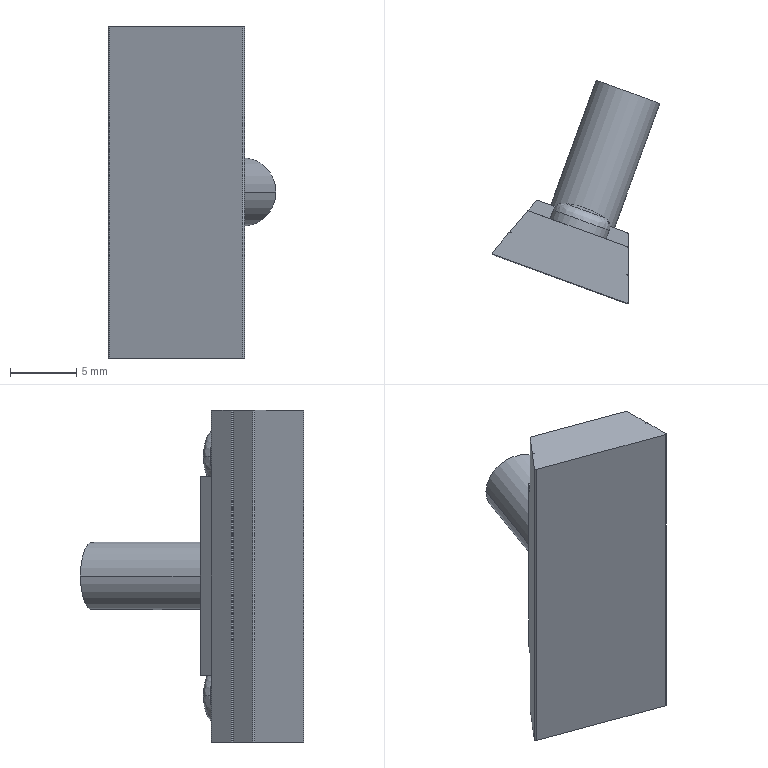Part | SolidWorks | features BaseBody 1 | 1 solid | 43 faces | box 12.626 x 16.806 x 25 mm | volume 1310 mm3 | plane 19 | cylinder 18 | spline 6 | commonest cylinder face diameters 0.2 x10 4.5 x4 5 x2 5.1 x2
STEP:
#1=CARTESIAN_POINT('',(0.2959,5.705,-9.));
#2=VERTEX_POINT('',#1);
#3=CARTESIAN_POINT('',(3.44,4.56,-9.));
#4=VERTEX_POINT('',#3);
#5=CARTESIAN_POINT('',(1.868,5.133,-9.));
#6=DIRECTION('',(-0.342,-0.9397,0.));
#7=DIRECTION('',(-0.9397,0.342,0.));
#8=AXIS2_PLACEMENT_3D('',#5,#6,#7);
#9=CIRCLE('',#8,1.673);
#10=EDGE_CURVE('',#2,#4,#9,.T.);
#11=ORIENTED_EDGE('',*,*,#10,.T.);
#12=CARTESIAN_POINT('',(3.72,3.641,-9.));
#13=VERTEX_POINT('',#12);
#14=CARTESIAN_POINT('',(2.968,3.915,-9.));
#15=DIRECTION('',(0.,0.,-1.));
#16=DIRECTION('',(0.9397,-0.342,0.));
#17=AXIS2_PLACEMENT_3D('',#14,#15,#16);
#18=CIRCLE('',#17,0.8);
#19=EDGE_CURVE('',#4,#13,#18,.T.);
#20=ORIENTED_EDGE('',*,*,#19,.T.);
#21=CARTESIAN_POINT('',(-0.509,5.18,-9.));
#22=VERTEX_POINT('',#21);
#23=CARTESIAN_POINT('',(1.605,4.411,-9.));
#24=DIRECTION('',(-0.342,-0.9397,0.));
#25=DIRECTION('',(0.9397,-0.342,0.));
#26=AXIS2_PLACEMENT_3D('',#23,#24,#25);
#27=CIRCLE('',#26,2.25);
#28=EDGE_CURVE('',#22,#13,#27,.T.);
#29=ORIENTED_EDGE('',*,*,#28,.F.);
#30=CARTESIAN_POINT('',(0.2428,4.907,-9.));
#31=DIRECTION('',(0.,0.,1.));
#32=DIRECTION('',(-0.9397,0.342,0.));
#33=AXIS2_PLACEMENT_3D('',#30,#31,#32);
#34=CIRCLE('',#33,0.8);
#35=EDGE_CURVE('',#2,#22,#34,.T.);
#36=ORIENTED_EDGE('',*,*,#35,.F.);
#37=EDGE_LOOP('',(#11,#20,#29,#36));
#38=FACE_OUTER_BOUND('',#37,.T.);
#39=CARTESIAN_POINT('',(3.44,4.56,-9.));
#40=CARTESIAN_POINT('',(3.44,4.56,-12.346));
#41=CARTESIAN_POINT('',(0.2959,5.705,-12.346));
#42=CARTESIAN_POINT('',(0.2959,5.705,-9.));
#43=CARTESIAN_POINT('',(3.739,4.342,-9.));
#44=CARTESIAN_POINT('',(3.739,4.342,-13.056));
#45=CARTESIAN_POINT('',(-0.07287,5.729,-13.056));
#46=CARTESIAN_POINT('',(-0.07287,5.729,-9.));
#47=CARTESIAN_POINT('',(3.846,3.988,-9.));
#48=CARTESIAN_POINT('',(3.846,3.988,-13.5));
#49=CARTESIAN_POINT('',(-0.3825,5.528,-13.5));
#50=CARTESIAN_POINT('',(-0.3825,5.528,-9.));
#51=CARTESIAN_POINT('',(3.72,3.641,-9.));
#52=CARTESIAN_POINT('',(3.72,3.641,-13.5));
#53=CARTESIAN_POINT('',(-0.509,5.18,-13.5));
#54=CARTESIAN_POINT('',(-0.509,5.18,-9.));
#55=(BOUNDED_SURFACE()B_SPLINE_SURFACE(3,3,((#39,#40,#41,#42),(#43,#44,#45,#46),(#47,#48,#49,#50),(#51,#52,#53,#54)),.UNSPECIFIED.,.F.,.F.,.T.)B_SPLINE_SURFACE_WITH_KNOTS((4,4),(4,4),(0.,1.),(0.,1.),.UNSPECIFIED.)GEOMETRIC_REPRESENTATION_ITEM()RATIONAL_B_SPLINE_SURFACE(((1.,0.3333,0.3333,1.),(0.8664,0.2888,0.2888,0.8664),(0.8664,0.2888,0.2888,0.8664),(1.,0.3333,0.3333,1.)))REPRESENTATION_ITEM('')SURFACE());
#56=ADVANCED_FACE('',(#38),#55,.T.);
#57=CARTESIAN_POINT('',(0.2959,5.705,9.));
#58=VERTEX_POINT('',#57);
#59=CARTESIAN_POINT('',(3.44,4.56,9.));
#60=VERTEX_POINT('',#59);
#61=CARTESIAN_POINT('',(1.868,5.133,9.));
#62=DIRECTION('',(-0.342,-0.9397,0.));
#63=DIRECTION('',(-0.9397,0.342,0.));
#64=AXIS2_PLACEMENT_3D('',#61,#62,#63);
#65=CIRCLE('',#64,1.673);
#66=EDGE_CURVE('',#58,#60,#65,.T.);
#67=ORIENTED_EDGE('',*,*,#66,.T.);
#68=CARTESIAN_POINT('',(3.72,3.641,9.));
#69=VERTEX_POINT('',#68);
#70=CARTESIAN_POINT('',(2.968,3.915,9.));
#71=DIRECTION('',(0.,0.,-1.));
#72=DIRECTION('',(0.9397,-0.342,0.));
#73=AXIS2_PLACEMENT_3D('',#70,#71,#72);
#74=CIRCLE('',#73,0.8);
#75=EDGE_CURVE('',#60,#69,#74,.T.);
#76=ORIENTED_EDGE('',*,*,#75,.T.);
#77=CARTESIAN_POINT('',(-0.509,5.18,9.));
#78=VERTEX_POINT('',#77);
#79=CARTESIAN_POINT('',(1.605,4.411,9.));
#80=DIRECTION('',(-0.342,-0.9397,0.));
#81=DIRECTION('',(0.9397,-0.342,0.));
#82=AXIS2_PLACEMENT_3D('',#79,#80,#81);
#83=CIRCLE('',#82,2.25);
#84=EDGE_CURVE('',#78,#69,#83,.T.);
#85=ORIENTED_EDGE('',*,*,#84,.F.);
#86=CARTESIAN_POINT('',(0.2428,4.907,9.));
#87=DIRECTION('',(0.,0.,1.));
#88=DIRECTION('',(-0.9397,0.342,0.));
#89=AXIS2_PLACEMENT_3D('',#86,#87,#88);
#90=CIRCLE('',#89,0.8);
#91=EDGE_CURVE('',#58,#78,#90,.T.);
#92=ORIENTED_EDGE('',*,*,#91,.F.);
#93=EDGE_LOOP('',(#67,#76,#85,#92));
#94=FACE_OUTER_BOUND('',#93,.T.);
#95=CARTESIAN_POINT('',(3.44,4.56,9.));
#96=CARTESIAN_POINT('',(3.44,4.56,5.654));
#97=CARTESIAN_POINT('',(0.2959,5.705,5.654));
#98=CARTESIAN_POINT('',(0.2959,5.705,9.));
#99=CARTESIAN_POINT('',(3.739,4.342,9.));
#100=CARTESIAN_POINT('',(3.739,4.342,4.944));
#101=CARTESIAN_POINT('',(-0.07287,5.729,4.944));
#102=CARTESIAN_POINT('',(-0.07287,5.729,9.));
#103=CARTESIAN_POINT('',(3.846,3.988,9.));
#104=CARTESIAN_POINT('',(3.846,3.988,4.5));
#105=CARTESIAN_POINT('',(-0.3825,5.528,4.5));
#106=CARTESIAN_POINT('',(-0.3825,5.528,9.));
#107=CARTESIAN_POINT('',(3.72,3.641,9.));
#108=CARTESIAN_POINT('',(3.72,3.641,4.5));
#109=CARTESIAN_POINT('',(-0.509,5.18,4.5));
#110=CARTESIAN_POINT('',(-0.509,5.18,9.));
#111=(BOUNDED_SURFACE()B_SPLINE_SURFACE(3,3,((#95,#96,#97,#98),(#99,#100,#101,#102),(#103,#104,#105,#106),(#107,#108,#109,#110)),.UNSPECIFIED.,.F.,.F.,.T.)B_SPLINE_SURFACE_WITH_KNOTS((4,4),(4,4),(0.,1.),(0.,1.),.UNSPECIFIED.)GEOMETRIC_REPRESENTATION_ITEM()RATIONAL_B_SPLINE_SURFACE(((1.,0.3333,0.3333,1.),(0.8664,0.2888,0.2888,0.8664),(0.8664,0.2888,0.2888,0.8664),(1.,0.3333,0.3333,1.)))REPRESENTATION_ITEM('')SURFACE());
#112=ADVANCED_FACE('',(#94),#111,.T.);
#113=CARTESIAN_POINT('',(1.605,4.411,-9.));
#114=DIRECTION('',(-0.342,-0.9397,0.));
#115=DIRECTION('',(0.9397,-0.342,0.));
#116=AXIS2_PLACEMENT_3D('',#113,#114,#115);
#117=CIRCLE('',#116,2.25);
#118=EDGE_CURVE('',#13,#22,#117,.T.);
#119=ORIENTED_EDGE('',*,*,#118,.T.);
#120=CARTESIAN_POINT('',(-0.7462,4.528,-9.));
#121=VERTEX_POINT('',#120);
#122=CARTESIAN_POINT('',(-0.1648,6.126,-9.));
#123=DIRECTION('',(-0.342,-0.9397,0.));
#124=VECTOR('',#123,1000.);
#125=LINE('',#122,#124);
#126=EDGE_CURVE('',#22,#121,#125,.T.);
#127=ORIENTED_EDGE('',*,*,#126,.T.);
#128=CARTESIAN_POINT('',(3.482,2.989,-9.));
#129=VERTEX_POINT('',#128);
#130=CARTESIAN_POINT('',(1.368,3.759,-9.));
#131=DIRECTION('',(0.342,0.9397,0.));
#132=DIRECTION('',(0.9397,-0.342,0.));
#133=AXIS2_PLACEMENT_3D('',#130,#131,#132);
#134=CIRCLE('',#133,2.25);
#135=EDGE_CURVE('',#121,#129,#134,.T.);
#136=ORIENTED_EDGE('',*,*,#135,.T.);
#137=CARTESIAN_POINT('',(4.064,4.587,-9.));
#138=DIRECTION('',(-0.342,-0.9397,0.));
#139=VECTOR('',#138,1000.);
#140=LINE('',#137,#139);
#141=EDGE_CURVE('',#13,#129,#140,.T.);
#142=ORIENTED_EDGE('',*,*,#141,.F.);
#143=EDGE_LOOP('',(#119,#127,#136,#142));
#144=FACE_OUTER_BOUND('',#143,.T.);
#145=CARTESIAN_POINT('',(1.95,5.356,-9.));
#146=DIRECTION('',(-0.342,-0.9397,0.));
#147=DIRECTION('',(0.9397,-0.342,0.));
#148=AXIS2_PLACEMENT_3D('',#145,#146,#147);
#149=CYLINDRICAL_SURFACE('',#148,2.25);
#150=ADVANCED_FACE('',(#144),#149,.T.);
#151=CARTESIAN_POINT('',(1.605,4.411,9.));
#152=DIRECTION('',(-0.342,-0.9397,0.));
#153=DIRECTION('',(0.9397,-0.342,0.));
#154=AXIS2_PLACEMENT_3D('',#151,#152,#153);
#155=CIRCLE('',#154,2.25);
#156=EDGE_CURVE('',#69,#78,#155,.T.);
#157=ORIENTED_EDGE('',*,*,#156,.T.);
#158=CARTESIAN_POINT('',(-0.7462,4.528,9.));
#159=VERTEX_POINT('',#158);
#160=CARTESIAN_POINT('',(-0.1648,6.126,9.));
#161=DIRECTION('',(-0.342,-0.9397,0.));
#162=VECTOR('',#161,1000.);
#163=LINE('',#160,#162);
#164=EDGE_CURVE('',#78,#159,#163,.T.);
#165=ORIENTED_EDGE('',*,*,#164,.T.);
#166=CARTESIAN_POINT('',(3.482,2.989,9.));
#167=VERTEX_POINT('',#166);
#168=CARTESIAN_POINT('',(1.368,3.759,9.));
#169=DIRECTION('',(0.342,0.9397,0.));
#170=DIRECTION('',(0.9397,-0.342,0.));
#171=AXIS2_PLACEMENT_3D('',#168,#169,#170);
#172=CIRCLE('',#171,2.25);
#173=EDGE_CURVE('',#159,#167,#172,.T.);
#174=ORIENTED_EDGE('',*,*,#173,.T.);
#175=CARTESIAN_POINT('',(4.064,4.587,9.));
#176=DIRECTION('',(-0.342,-0.9397,0.));
#177=VECTOR('',#176,1000.);
#178=LINE('',#175,#177);
#179=EDGE_CURVE('',#69,#167,#178,.T.);
#180=ORIENTED_EDGE('',*,*,#179,.F.);
#181=EDGE_LOOP('',(#157,#165,#174,#180));
#182=FACE_OUTER_BOUND('',#181,.T.);
#183=CARTESIAN_POINT('',(1.95,5.356,9.));
#184=DIRECTION('',(-0.342,-0.9397,0.));
#185=DIRECTION('',(0.9397,-0.342,0.));
#186=AXIS2_PLACEMENT_3D('',#183,#184,#185);
#187=CYLINDRICAL_SURFACE('',#186,2.25);
#188=ADVANCED_FACE('',(#182),#187,.T.);
#189=CARTESIAN_POINT('',(-0.6861,5.571,0.));
#190=VERTEX_POINT('',#189);
#191=CARTESIAN_POINT('',(4.106,3.826,0.));
#192=VERTEX_POINT('',#191);
#193=CARTESIAN_POINT('',(1.71,4.698,0.));
#194=DIRECTION('',(0.342,0.9397,0.));
#195=DIRECTION('',(-0.9397,0.342,0.));
#196=AXIS2_PLACEMENT_3D('',#193,#194,#195);
#197=CIRCLE('',#196,2.55);
#198=EDGE_CURVE('',#190,#192,#197,.T.);
#199=ORIENTED_EDGE('',*,*,#198,.T.);
#200=CARTESIAN_POINT('',(7.527,13.223,0.));
#201=VERTEX_POINT('',#200);
#202=CARTESIAN_POINT('',(7.527,13.223,0.));
#203=DIRECTION('',(0.342,0.9397,0.));
#204=VECTOR('',#203,1000.);
#205=LINE('',#202,#204);
#206=EDGE_CURVE('',#192,#201,#205,.T.);
#207=ORIENTED_EDGE('',*,*,#206,.T.);
#208=CARTESIAN_POINT('',(2.734,14.968,0.));
#209=VERTEX_POINT('',#208);
#210=CARTESIAN_POINT('',(5.13,14.095,0.));
#211=DIRECTION('',(-0.342,-0.9397,0.));
#212=DIRECTION('',(-0.9397,0.342,0.));
#213=AXIS2_PLACEMENT_3D('',#210,#211,#212);
#214=CIRCLE('',#213,2.55);
#215=EDGE_CURVE('',#201,#209,#214,.T.);
#216=ORIENTED_EDGE('',*,*,#215,.T.);
#217=CARTESIAN_POINT('',(2.734,14.968,0.));
#218=DIRECTION('',(0.342,0.9397,0.));
#219=VECTOR('',#218,1000.);
#220=LINE('',#217,#219);
#221=EDGE_CURVE('',#190,#209,#220,.T.);
#222=ORIENTED_EDGE('',*,*,#221,.F.);
#223=EDGE_LOOP('',(#199,#207,#216,#222));
#224=FACE_OUTER_BOUND('',#223,.T.);
#225=CARTESIAN_POINT('',(5.13,14.095,0.));
#226=DIRECTION('',(0.342,0.9397,0.));
#227=DIRECTION('',(-0.9397,0.342,0.));
#228=AXIS2_PLACEMENT_3D('',#225,#226,#227);
#229=CYLINDRICAL_SURFACE('',#228,2.55);
#230=ADVANCED_FACE('',(#224),#229,.T.);
#231=CARTESIAN_POINT('',(5.034,-1.832,12.5));
#232=VERTEX_POINT('',#231);
#233=CARTESIAN_POINT('',(5.034,-1.832,-12.5));
#234=VERTEX_POINT('',#233);
#235=CARTESIAN_POINT('',(5.034,-1.832,12.5));
#236=DIRECTION('',(0.,0.,-1.));
#237=VECTOR('',#236,1000.);
#238=LINE('',#235,#237);
#239=EDGE_CURVE('',#232,#234,#238,.T.);
#240=ORIENTED_EDGE('',*,*,#239,.F.);
#241=CARTESIAN_POINT('',(-5.034,1.832,12.5));
#242=VERTEX_POINT('',#241);
#243=CARTESIAN_POINT('',(-5.034,1.832,12.5));
#244=DIRECTION('',(0.9397,-0.342,0.));
#245=VECTOR('',#244,1000.);
#246=LINE('',#243,#245);
#247=EDGE_CURVE('',#242,#232,#246,.T.);
#248=ORIENTED_EDGE('',*,*,#247,.F.);
#249=CARTESIAN_POINT('',(-5.034,1.832,-12.5));
#250=VERTEX_POINT('',#249);
#251=CARTESIAN_POINT('',(-5.034,1.832,12.5));
#252=DIRECTION('',(0.,0.,1.));
#253=VECTOR('',#252,1000.);
#254=LINE('',#251,#253);
#255=EDGE_CURVE('',#250,#242,#254,.T.);
#256=ORIENTED_EDGE('',*,*,#255,.F.);
#257=CARTESIAN_POINT('',(-5.034,1.832,-12.5));
#258=DIRECTION('',(-0.9397,0.342,0.));
#259=VECTOR('',#258,1000.);
#260=LINE('',#257,#259);
#261=EDGE_CURVE('',#234,#250,#260,.T.);
#262=ORIENTED_EDGE('',*,*,#261,.F.);
#263=EDGE_LOOP('',(#240,#248,#256,#262));
#264=FACE_OUTER_BOUND('',#263,.T.);
#265=CARTESIAN_POINT('',(-5.034,1.832,12.5));
#266=DIRECTION('',(0.342,0.9397,0.));
#267=DIRECTION('',(-0.9397,0.342,0.));
#268=AXIS2_PLACEMENT_3D('',#265,#266,#267);
#269=PLANE('',#268);
#270=ADVANCED_FACE('',(#264),#269,.F.);
#271=CARTESIAN_POINT('',(-3.734,3.488,-12.5));
#272=VERTEX_POINT('',#271);
#273=CARTESIAN_POINT('',(-3.845,3.458,-12.5));
#274=VERTEX_POINT('',#273);
#275=CARTESIAN_POINT('',(-3.769,3.394,-12.5));
#276=DIRECTION('',(0.,0.,1.));
#277=DIRECTION('',(1.,0.,0.));
#278=AXIS2_PLACEMENT_3D('',#275,#276,#277);
#279=CIRCLE('',#278,0.1);
#280=EDGE_CURVE('',#272,#274,#279,.T.);
#281=ORIENTED_EDGE('',*,*,#280,.F.);
#282=CARTESIAN_POINT('',(-3.643,3.454,-12.5));
#283=VERTEX_POINT('',#282);
#284=CARTESIAN_POINT('',(5.103,0.2712,-12.5));
#285=DIRECTION('',(0.9397,-0.342,0.));
#286=VECTOR('',#285,1000.);
#287=LINE('',#284,#286);
#288=EDGE_CURVE('',#272,#283,#287,.T.);
#289=ORIENTED_EDGE('',*,*,#288,.T.);
#290=CARTESIAN_POINT('',(-3.685,3.613,-12.5));
#291=VERTEX_POINT('',#290);
#292=CARTESIAN_POINT('',(-3.609,3.548,-12.5));
#293=DIRECTION('',(0.,0.,1.));
#294=DIRECTION('',(1.,0.,0.));
#295=AXIS2_PLACEMENT_3D('',#292,#293,#294);
#296=CIRCLE('',#295,0.1);
#297=EDGE_CURVE('',#291,#283,#296,.T.);
#298=ORIENTED_EDGE('',*,*,#297,.F.);
#299=CARTESIAN_POINT('',(-2.454,5.08,-12.5));
#300=VERTEX_POINT('',#299);
#301=CARTESIAN_POINT('',(-2.454,5.08,-12.5));
#302=DIRECTION('',(-0.6428,-0.766,0.));
#303=VECTOR('',#302,1000.);
#304=LINE('',#301,#303);
#305=EDGE_CURVE('',#300,#291,#304,.T.);
#306=ORIENTED_EDGE('',*,*,#305,.F.);
#307=CARTESIAN_POINT('',(-2.343,5.11,-12.5));
#308=VERTEX_POINT('',#307);
#309=CARTESIAN_POINT('',(-2.377,5.016,-12.5));
#310=DIRECTION('',(0.,0.,1.));
#311=DIRECTION('',(1.,0.,0.));
#312=AXIS2_PLACEMENT_3D('',#309,#310,#311);
#313=CIRCLE('',#312,0.1);
#314=EDGE_CURVE('',#308,#300,#313,.T.);
#315=ORIENTED_EDGE('',*,*,#314,.F.);
#316=CARTESIAN_POINT('',(5.079,2.408,-12.5));
#317=VERTEX_POINT('',#316);
#318=CARTESIAN_POINT('',(5.079,2.408,-12.5));
#319=DIRECTION('',(-0.9397,0.342,0.));
#320=VECTOR('',#319,1000.);
#321=LINE('',#318,#320);
#322=EDGE_CURVE('',#317,#308,#321,.T.);
#323=ORIENTED_EDGE('',*,*,#322,.F.);
#324=CARTESIAN_POINT('',(5.145,2.314,-12.5));
#325=VERTEX_POINT('',#324);
#326=CARTESIAN_POINT('',(5.045,2.314,-12.5));
#327=DIRECTION('',(0.,0.,1.));
#328=DIRECTION('',(1.,0.,0.));
#329=AXIS2_PLACEMENT_3D('',#326,#327,#328);
#330=CIRCLE('',#329,0.1);
#331=EDGE_CURVE('',#325,#317,#330,.T.);
#332=ORIENTED_EDGE('',*,*,#331,.F.);
#333=CARTESIAN_POINT('',(5.145,0.3985,-12.5));
#334=VERTEX_POINT('',#333);
#335=CARTESIAN_POINT('',(5.145,1.926,-12.5));
#336=DIRECTION('',(0.,1.,0.));
#337=VECTOR('',#336,1000.);
#338=LINE('',#335,#337);
#339=EDGE_CURVE('',#334,#325,#338,.T.);
#340=ORIENTED_EDGE('',*,*,#339,.F.);
#341=CARTESIAN_POINT('',(5.011,0.3045,-12.5));
#342=VERTEX_POINT('',#341);
#343=CARTESIAN_POINT('',(5.045,0.3985,-12.5));
#344=DIRECTION('',(0.,0.,1.));
#345=DIRECTION('',(1.,0.,0.));
#346=AXIS2_PLACEMENT_3D('',#343,#344,#345);
#347=CIRCLE('',#346,0.1);
#348=EDGE_CURVE('',#342,#334,#347,.T.);
#349=ORIENTED_EDGE('',*,*,#348,.F.);
#350=CARTESIAN_POINT('',(5.103,0.2712,-12.5));
#351=VERTEX_POINT('',#350);
#352=CARTESIAN_POINT('',(5.103,0.2712,-12.5));
#353=DIRECTION('',(0.9397,-0.342,0.));
#354=VECTOR('',#353,1000.);
#355=LINE('',#352,#354);
#356=EDGE_CURVE('',#342,#351,#355,.T.);
#357=ORIENTED_EDGE('',*,*,#356,.T.);
#358=CARTESIAN_POINT('',(5.168,0.1772,-12.5));
#359=VERTEX_POINT('',#358);
#360=CARTESIAN_POINT('',(5.068,0.1772,-12.5));
#361=DIRECTION('',(0.,0.,1.));
#362=DIRECTION('',(1.,0.,0.));
#363=AXIS2_PLACEMENT_3D('',#360,#361,#362);
#364=CIRCLE('',#363,0.1);
#365=EDGE_CURVE('',#359,#351,#364,.T.);
#366=ORIENTED_EDGE('',*,*,#365,.F.);
#367=CARTESIAN_POINT('',(5.168,-1.738,-12.5));
#368=VERTEX_POINT('',#367);
#369=CARTESIAN_POINT('',(5.168,1.926,-12.5));
#370=DIRECTION('',(0.,1.,0.));
#371=VECTOR('',#370,1000.);
#372=LINE('',#369,#371);
#373=EDGE_CURVE('',#368,#359,#372,.T.);
#374=ORIENTED_EDGE('',*,*,#373,.F.);
#375=CARTESIAN_POINT('',(5.068,-1.738,-12.5));
#376=DIRECTION('',(0.,0.,1.));
#377=DIRECTION('',(1.,0.,0.));
#378=AXIS2_PLACEMENT_3D('',#375,#376,#377);
#379=CIRCLE('',#378,0.1);
#380=EDGE_CURVE('',#234,#368,#379,.T.);
#381=ORIENTED_EDGE('',*,*,#380,.F.);
#382=ORIENTED_EDGE('',*,*,#261,.T.);
#383=CARTESIAN_POINT('',(-5.077,1.991,-12.5));
#384=VERTEX_POINT('',#383);
#385=CARTESIAN_POINT('',(-5.,1.926,-12.5));
#386=DIRECTION('',(0.,0.,1.));
#387=DIRECTION('',(1.,0.,0.));
#388=AXIS2_PLACEMENT_3D('',#385,#386,#387);
#389=CIRCLE('',#388,0.1);
#390=EDGE_CURVE('',#384,#250,#389,.T.);
#391=ORIENTED_EDGE('',*,*,#390,.F.);
#392=CARTESIAN_POINT('',(-3.845,3.458,-12.5));
#393=DIRECTION('',(-0.6428,-0.766,0.));
#394=VECTOR('',#393,1000.);
#395=LINE('',#392,#394);
#396=EDGE_CURVE('',#274,#384,#395,.T.);
#397=ORIENTED_EDGE('',*,*,#396,.F.);
#398=EDGE_LOOP('',(#281,#289,#298,#306,#315,#323,#332,#340,#349,#357,#366,#374,#381,#382,#391,#397));
#399=FACE_OUTER_BOUND('',#398,.T.);
#400=CARTESIAN_POINT('',(-5.,1.926,-12.5));
#401=DIRECTION('',(0.,0.,1.));
#402=DIRECTION('',(1.,0.,0.));
#403=AXIS2_PLACEMENT_3D('',#400,#401,#402);
#404=PLANE('',#403);
#405=ADVANCED_FACE('',(#399),#404,.F.);
#406=CARTESIAN_POINT('',(5.168,-1.738,12.5));
#407=VERTEX_POINT('',#406);
#408=CARTESIAN_POINT('',(5.068,-1.738,12.5));
#409=DIRECTION('',(0.,0.,-1.));
#410=DIRECTION('',(1.,0.,0.));
#411=AXIS2_PLACEMENT_3D('',#408,#409,#410);
#412=CIRCLE('',#411,0.1);
#413=EDGE_CURVE('',#407,#232,#412,.T.);
#414=ORIENTED_EDGE('',*,*,#413,.T.);
#415=ORIENTED_EDGE('',*,*,#239,.T.);
#416=ORIENTED_EDGE('',*,*,#380,.T.);
#417=CARTESIAN_POINT('',(5.168,-1.738,12.5));
#418=DIRECTION('',(0.,0.,1.));
#419=VECTOR('',#418,1000.);
#420=LINE('',#417,#419);
#421=EDGE_CURVE('',#368,#407,#420,.T.);
#422=ORIENTED_EDGE('',*,*,#421,.T.);
#423=EDGE_LOOP('',(#414,#415,#416,#422));
#424=FACE_OUTER_BOUND('',#423,.T.);
#425=CARTESIAN_POINT('',(5.068,-1.738,12.5));
#426=DIRECTION('',(0.,0.,1.));
#427=DIRECTION('',(1.,0.,0.));
#428=AXIS2_PLACEMENT_3D('',#425,#426,#427);
#429=CYLINDRICAL_SURFACE('',#428,0.1);
#430=ADVANCED_FACE('',(#424),#429,.T.);
#431=CARTESIAN_POINT('',(-3.643,3.454,12.5));
#432=VERTEX_POINT('',#431);
#433=CARTESIAN_POINT('',(-3.734,3.488,12.5));
#434=VERTEX_POINT('',#433);
#435=CARTESIAN_POINT('',(5.103,0.2712,12.5));
#436=DIRECTION('',(-0.9397,0.342,0.));
#437=VECTOR('',#436,1000.);
#438=LINE('',#435,#437);
#439=EDGE_CURVE('',#432,#434,#438,.T.);
#440=ORIENTED_EDGE('',*,*,#439,.T.);
#441=CARTESIAN_POINT('',(-3.845,3.458,12.5));
#442=VERTEX_POINT('',#441);
#443=CARTESIAN_POINT('',(-3.769,3.394,12.5));
#444=DIRECTION('',(0.,0.,-1.));
#445=DIRECTION('',(1.,0.,0.));
#446=AXIS2_PLACEMENT_3D('',#443,#444,#445);
#447=CIRCLE('',#446,0.1);
#448=EDGE_CURVE('',#442,#434,#447,.T.);
#449=ORIENTED_EDGE('',*,*,#448,.F.);
#450=CARTESIAN_POINT('',(-5.077,1.991,12.5));
#451=VERTEX_POINT('',#450);
#452=CARTESIAN_POINT('',(-3.845,3.458,12.5));
#453=DIRECTION('',(-0.6428,-0.766,0.));
#454=VECTOR('',#453,1000.);
#455=LINE('',#452,#454);
#456=EDGE_CURVE('',#442,#451,#455,.T.);
#457=ORIENTED_EDGE('',*,*,#456,.T.);
#458=CARTESIAN_POINT('',(-5.,1.926,12.5));
#459=DIRECTION('',(0.,0.,1.));
#460=DIRECTION('',(1.,0.,0.));
#461=AXIS2_PLACEMENT_3D('',#458,#459,#460);
#462=CIRCLE('',#461,0.1);
#463=EDGE_CURVE('',#451,#242,#462,.T.);
#464=ORIENTED_EDGE('',*,*,#463,.T.);
#465=ORIENTED_EDGE('',*,*,#247,.T.);
#466=ORIENTED_EDGE('',*,*,#413,.F.);
#467=CARTESIAN_POINT('',(5.168,0.1772,12.5));
#468=VERTEX_POINT('',#467);
#469=CARTESIAN_POINT('',(5.168,1.926,12.5));
#470=DIRECTION('',(0.,1.,0.));
#471=VECTOR('',#470,1000.);
#472=LINE('',#469,#471);
#473=EDGE_CURVE('',#407,#468,#472,.T.);
#474=ORIENTED_EDGE('',*,*,#473,.T.);
#475=CARTESIAN_POINT('',(5.103,0.2712,12.5));
#476=VERTEX_POINT('',#475);
#477=CARTESIAN_POINT('',(5.068,0.1772,12.5));
#478=DIRECTION('',(0.,0.,-1.));
#479=DIRECTION('',(1.,0.,0.));
#480=AXIS2_PLACEMENT_3D('',#477,#478,#479);
#481=CIRCLE('',#480,0.1);
#482=EDGE_CURVE('',#476,#468,#481,.T.);
#483=ORIENTED_EDGE('',*,*,#482,.F.);
#484=CARTESIAN_POINT('',(5.011,0.3045,12.5));
#485=VERTEX_POINT('',#484);
#486=CARTESIAN_POINT('',(5.103,0.2712,12.5));
#487=DIRECTION('',(-0.9397,0.342,0.));
#488=VECTOR('',#487,1000.);
#489=LINE('',#486,#488);
#490=EDGE_CURVE('',#476,#485,#489,.T.);
#491=ORIENTED_EDGE('',*,*,#490,.T.);
#492=CARTESIAN_POINT('',(5.145,0.3985,12.5));
#493=VERTEX_POINT('',#492);
#494=CARTESIAN_POINT('',(5.045,0.3985,12.5));
#495=DIRECTION('',(0.,0.,-1.));
#496=DIRECTION('',(1.,0.,0.));
#497=AXIS2_PLACEMENT_3D('',#494,#495,#496);
#498=CIRCLE('',#497,0.1);
#499=EDGE_CURVE('',#493,#485,#498,.T.);
#500=ORIENTED_EDGE('',*,*,#499,.F.);
#501=CARTESIAN_POINT('',(5.145,2.314,12.5));
#502=VERTEX_POINT('',#501);
#503=CARTESIAN_POINT('',(5.145,1.926,12.5));
#504=DIRECTION('',(0.,1.,0.));
#505=VECTOR('',#504,1000.);
#506=LINE('',#503,#505);
#507=EDGE_CURVE('',#493,#502,#506,.T.);
#508=ORIENTED_EDGE('',*,*,#507,.T.);
#509=CARTESIAN_POINT('',(5.079,2.408,12.5));
#510=VERTEX_POINT('',#509);
#511=CARTESIAN_POINT('',(5.045,2.314,12.5));
#512=DIRECTION('',(0.,0.,-1.));
#513=DIRECTION('',(1.,0.,0.));
#514=AXIS2_PLACEMENT_3D('',#511,#512,#513);
#515=CIRCLE('',#514,0.1);
#516=EDGE_CURVE('',#510,#502,#515,.T.);
#517=ORIENTED_EDGE('',*,*,#516,.F.);
#518=CARTESIAN_POINT('',(-2.343,5.11,12.5));
#519=VERTEX_POINT('',#518);
#520=CARTESIAN_POINT('',(5.079,2.408,12.5));
#521=DIRECTION('',(-0.9397,0.342,0.));
#522=VECTOR('',#521,1000.);
#523=LINE('',#520,#522);
#524=EDGE_CURVE('',#510,#519,#523,.T.);
#525=ORIENTED_EDGE('',*,*,#524,.T.);
#526=CARTESIAN_POINT('',(-2.454,5.08,12.5));
#527=VERTEX_POINT('',#526);
#528=CARTESIAN_POINT('',(-2.377,5.016,12.5));
#529=DIRECTION('',(0.,0.,-1.));
#530=DIRECTION('',(1.,0.,0.));
#531=AXIS2_PLACEMENT_3D('',#528,#529,#530);
#532=CIRCLE('',#531,0.1);
#533=EDGE_CURVE('',#527,#519,#532,.T.);
#534=ORIENTED_EDGE('',*,*,#533,.F.);
#535=CARTESIAN_POINT('',(-3.685,3.613,12.5));
#536=VERTEX_POINT('',#535);
#537=CARTESIAN_POINT('',(-2.454,5.08,12.5));
#538=DIRECTION('',(-0.6428,-0.766,0.));
#539=VECTOR('',#538,1000.);
#540=LINE('',#537,#539);
#541=EDGE_CURVE('',#527,#536,#540,.T.);
#542=ORIENTED_EDGE('',*,*,#541,.T.);
#543=CARTESIAN_POINT('',(-3.609,3.548,12.5));
#544=DIRECTION('',(0.,0.,-1.));
#545=DIRECTION('',(1.,0.,0.));
#546=AXIS2_PLACEMENT_3D('',#543,#544,#545);
#547=CIRCLE('',#546,0.1);
#548=EDGE_CURVE('',#432,#536,#547,.T.);
#549=ORIENTED_EDGE('',*,*,#548,.F.);
#550=EDGE_LOOP('',(#440,#449,#457,#464,#465,#466,#474,#483,#491,#500,#508,#517,#525,#534,#542,#549));
#551=FACE_OUTER_BOUND('',#550,.T.);
#552=CARTESIAN_POINT('',(-5.,1.926,12.5));
#553=DIRECTION('',(0.,0.,1.));
#554=DIRECTION('',(1.,0.,0.));
#555=AXIS2_PLACEMENT_3D('',#552,#553,#554);
#556=PLANE('',#555);
#557=ADVANCED_FACE('',(#551),#556,.T.);
#558=ORIENTED_EDGE('',*,*,#463,.F.);
#559=CARTESIAN_POINT('',(-5.077,1.991,12.5));
#560=DIRECTION('',(0.,0.,-1.));
#561=VECTOR('',#560,1000.);
#562=LINE('',#559,#561);
#563=EDGE_CURVE('',#451,#384,#562,.T.);
#564=ORIENTED_EDGE('',*,*,#563,.T.);
#565=ORIENTED_EDGE('',*,*,#390,.T.);
#566=ORIENTED_EDGE('',*,*,#255,.T.);
#567=EDGE_LOOP('',(#558,#564,#565,#566));
#568=FACE_OUTER_BOUND('',#567,.T.);
#569=CARTESIAN_POINT('',(-5.,1.926,12.5));
#570=DIRECTION('',(0.,0.,1.));
#571=DIRECTION('',(1.,0.,0.));
#572=AXIS2_PLACEMENT_3D('',#569,#570,#571);
#573=CYLINDRICAL_SURFACE('',#572,0.1);
#574=ADVANCED_FACE('',(#568),#573,.T.);
#575=ORIENTED_EDGE('',*,*,#563,.F.);
#576=ORIENTED_EDGE('',*,*,#456,.F.);
#577=CARTESIAN_POINT('',(-3.845,3.458,12.5));
#578=DIRECTION('',(0.,0.,1.));
#579=VECTOR('',#578,1000.);
#580=LINE('',#577,#579);
#581=EDGE_CURVE('',#274,#442,#580,.T.);
#582=ORIENTED_EDGE('',*,*,#581,.F.);
#583=ORIENTED_EDGE('',*,*,#396,.T.);
#584=EDGE_LOOP('',(#575,#576,#582,#583));
#585=FACE_OUTER_BOUND('',#584,.T.);
#586=CARTESIAN_POINT('',(-3.845,3.458,12.5));
#587=DIRECTION('',(0.766,-0.6428,0.));
#588=DIRECTION('',(0.6428,0.766,0.));
#589=AXIS2_PLACEMENT_3D('',#586,#587,#588);
#590=PLANE('',#589);
#591=ADVANCED_FACE('',(#585),#590,.F.);
#592=CARTESIAN_POINT('',(-3.685,3.613,12.5));
#593=DIRECTION('',(0.,0.,-1.));
#594=VECTOR('',#593,1000.);
#595=LINE('',#592,#594);
#596=EDGE_CURVE('',#536,#291,#595,.T.);
#597=ORIENTED_EDGE('',*,*,#596,.F.);
#598=ORIENTED_EDGE('',*,*,#541,.F.);
#599=CARTESIAN_POINT('',(-2.454,5.08,12.5));
#600=DIRECTION('',(0.,0.,1.));
#601=VECTOR('',#600,1000.);
#602=LINE('',#599,#601);
#603=EDGE_CURVE('',#300,#527,#602,.T.);
#604=ORIENTED_EDGE('',*,*,#603,.F.);
#605=ORIENTED_EDGE('',*,*,#305,.T.);
#606=EDGE_LOOP('',(#597,#598,#604,#605));
#607=FACE_OUTER_BOUND('',#606,.T.);
#608=CARTESIAN_POINT('',(-2.454,5.08,12.5));
#609=DIRECTION('',(0.766,-0.6428,0.));
#610=DIRECTION('',(0.6428,0.766,0.));
#611=AXIS2_PLACEMENT_3D('',#608,#609,#610);
#612=PLANE('',#611);
#613=ADVANCED_FACE('',(#607),#612,.F.);
#614=CARTESIAN_POINT('',(3.219,3.085,-7.46));
#615=VERTEX_POINT('',#614);
#616=CARTESIAN_POINT('',(-0.4827,4.432,-7.46));
#617=VERTEX_POINT('',#616);
#618=CARTESIAN_POINT('',(1.368,3.759,-9.));
#619=DIRECTION('',(-0.342,-0.9397,0.));
#620=DIRECTION('',(-0.9397,0.342,0.));
#621=AXIS2_PLACEMENT_3D('',#618,#619,#620);
#622=CIRCLE('',#621,2.5);
#623=EDGE_CURVE('',#615,#617,#622,.T.);
#624=ORIENTED_EDGE('',*,*,#623,.F.);
#625=CARTESIAN_POINT('',(5.079,2.408,-7.46));
#626=VERTEX_POINT('',#625);
#627=CARTESIAN_POINT('',(5.079,2.408,-7.46));
#628=DIRECTION('',(-0.9397,0.342,0.));
#629=VECTOR('',#628,1000.);
#630=LINE('',#627,#629);
#631=EDGE_CURVE('',#626,#615,#630,.T.);
#632=ORIENTED_EDGE('',*,*,#631,.F.);
#633=CARTESIAN_POINT('',(5.079,2.408,12.5));
#634=DIRECTION('',(0.,0.,1.));
#635=VECTOR('',#634,1000.);
#636=LINE('',#633,#635);
#637=EDGE_CURVE('',#317,#626,#636,.T.);
#638=ORIENTED_EDGE('',*,*,#637,.F.);
#639=ORIENTED_EDGE('',*,*,#322,.T.);
#640=CARTESIAN_POINT('',(-2.343,5.11,-7.46));
#641=VERTEX_POINT('',#640);
#642=CARTESIAN_POINT('',(-2.343,5.11,12.5));
#643=DIRECTION('',(0.,0.,-1.));
#644=VECTOR('',#643,1000.);
#645=LINE('',#642,#644);
#646=EDGE_CURVE('',#641,#308,#645,.T.);
#647=ORIENTED_EDGE('',*,*,#646,.F.);
#648=CARTESIAN_POINT('',(5.079,2.408,-7.46));
#649=DIRECTION('',(-0.9397,0.342,0.));
#650=VECTOR('',#649,1000.);
#651=LINE('',#648,#650);
#652=EDGE_CURVE('',#617,#641,#651,.T.);
#653=ORIENTED_EDGE('',*,*,#652,.F.);
#654=EDGE_LOOP('',(#624,#632,#638,#639,#647,#653));
#655=FACE_OUTER_BOUND('',#654,.T.);
#656=CARTESIAN_POINT('',(1.368,3.759,-9.));
#657=DIRECTION('',(0.342,0.9397,0.));
#658=DIRECTION('',(0.9397,-0.342,0.));
#659=AXIS2_PLACEMENT_3D('',#656,#657,#658);
#660=CIRCLE('',#659,2.25);
#661=EDGE_CURVE('',#129,#121,#660,.T.);
#662=ORIENTED_EDGE('',*,*,#661,.F.);
#663=ORIENTED_EDGE('',*,*,#135,.F.);
#664=EDGE_LOOP('',(#662,#663));
#665=FACE_BOUND('',#664,.T.);
#666=CARTESIAN_POINT('',(5.079,2.408,12.5));
#667=DIRECTION('',(-0.342,-0.9397,0.));
#668=DIRECTION('',(0.9397,-0.342,0.));
#669=AXIS2_PLACEMENT_3D('',#666,#667,#668);
#670=PLANE('',#669);
#671=ADVANCED_FACE('',(#655,#665),#670,.F.);
#672=CARTESIAN_POINT('',(5.145,2.314,12.5));
#673=DIRECTION('',(0.,0.,-1.));
#674=VECTOR('',#673,1000.);
#675=LINE('',#672,#674);
#676=EDGE_CURVE('',#502,#325,#675,.T.);
#677=ORIENTED_EDGE('',*,*,#676,.F.);
#678=ORIENTED_EDGE('',*,*,#507,.F.);
#679=CARTESIAN_POINT('',(5.145,0.3985,12.5));
#680=DIRECTION('',(0.,0.,1.));
#681=VECTOR('',#680,1000.);
#682=LINE('',#679,#681);
#683=EDGE_CURVE('',#334,#493,#682,.T.);
#684=ORIENTED_EDGE('',*,*,#683,.F.);
#685=ORIENTED_EDGE('',*,*,#339,.T.);
#686=EDGE_LOOP('',(#677,#678,#684,#685));
#687=FACE_OUTER_BOUND('',#686,.T.);
#688=CARTESIAN_POINT('',(5.145,0.3985,12.5));
#689=DIRECTION('',(-1.,0.,0.));
#690=DIRECTION('',(0.,-1.,0.));
#691=AXIS2_PLACEMENT_3D('',#688,#689,#690);
#692=PLANE('',#691);
#693=ADVANCED_FACE('',(#687),#692,.F.);
#694=CARTESIAN_POINT('',(5.168,0.1772,12.5));
#695=DIRECTION('',(0.,0.,-1.));
#696=VECTOR('',#695,1000.);
#697=LINE('',#694,#696);
#698=EDGE_CURVE('',#468,#359,#697,.T.);
#699=ORIENTED_EDGE('',*,*,#698,.F.);
#700=ORIENTED_EDGE('',*,*,#473,.F.);
#701=ORIENTED_EDGE('',*,*,#421,.F.);
#702=ORIENTED_EDGE('',*,*,#373,.T.);
#703=EDGE_LOOP('',(#699,#700,#701,#702));
#704=FACE_OUTER_BOUND('',#703,.T.);
#705=CARTESIAN_POINT('',(5.168,-1.738,12.5));
#706=DIRECTION('',(-1.,0.,0.));
#707=DIRECTION('',(0.,-1.,0.));
#708=AXIS2_PLACEMENT_3D('',#705,#706,#707);
#709=PLANE('',#708);
#710=ADVANCED_FACE('',(#704),#709,.F.);
#711=CARTESIAN_POINT('',(-0.4827,4.432,7.46));
#712=VERTEX_POINT('',#711);
#713=CARTESIAN_POINT('',(3.219,3.085,7.46));
#714=VERTEX_POINT('',#713);
#715=CARTESIAN_POINT('',(1.368,3.759,9.));
#716=DIRECTION('',(-0.342,-0.9397,0.));
#717=DIRECTION('',(-0.9397,0.342,0.));
#718=AXIS2_PLACEMENT_3D('',#715,#716,#717);
#719=CIRCLE('',#718,2.5);
#720=EDGE_CURVE('',#712,#714,#719,.T.);
#721=ORIENTED_EDGE('',*,*,#720,.F.);
#722=CARTESIAN_POINT('',(-2.343,5.11,7.46));
#723=VERTEX_POINT('',#722);
#724=CARTESIAN_POINT('',(5.079,2.408,7.46));
#725=DIRECTION('',(0.9397,-0.342,0.));
#726=VECTOR('',#725,1000.);
#727=LINE('',#724,#726);
#728=EDGE_CURVE('',#723,#712,#727,.T.);
#729=ORIENTED_EDGE('',*,*,#728,.F.);
#730=CARTESIAN_POINT('',(-2.343,5.11,12.5));
#731=DIRECTION('',(0.,0.,-1.));
#732=VECTOR('',#731,1000.);
#733=LINE('',#730,#732);
#734=EDGE_CURVE('',#519,#723,#733,.T.);
#735=ORIENTED_EDGE('',*,*,#734,.F.);
#736=ORIENTED_EDGE('',*,*,#524,.F.);
#737=CARTESIAN_POINT('',(5.079,2.408,7.46));
#738=VERTEX_POINT('',#737);
#739=CARTESIAN_POINT('',(5.079,2.408,12.5));
#740=DIRECTION('',(0.,0.,1.));
#741=VECTOR('',#740,1000.);
#742=LINE('',#739,#741);
#743=EDGE_CURVE('',#738,#510,#742,.T.);
#744=ORIENTED_EDGE('',*,*,#743,.F.);
#745=CARTESIAN_POINT('',(5.079,2.408,7.46));
#746=DIRECTION('',(0.9397,-0.342,0.));
#747=VECTOR('',#746,1000.);
#748=LINE('',#745,#747);
#749=EDGE_CURVE('',#714,#738,#748,.T.);
#750=ORIENTED_EDGE('',*,*,#749,.F.);
#751=EDGE_LOOP('',(#721,#729,#735,#736,#744,#750));
#752=FACE_OUTER_BOUND('',#751,.T.);
#753=CARTESIAN_POINT('',(1.368,3.759,9.));
#754=DIRECTION('',(0.342,0.9397,0.));
#755=DIRECTION('',(0.9397,-0.342,0.));
#756=AXIS2_PLACEMENT_3D('',#753,#754,#755);
#757=CIRCLE('',#756,2.25);
#758=EDGE_CURVE('',#167,#159,#757,.T.);
#759=ORIENTED_EDGE('',*,*,#758,.F.);
#760=ORIENTED_EDGE('',*,*,#173,.F.);
#761=EDGE_LOOP('',(#759,#760));
#762=FACE_BOUND('',#761,.T.);
#763=CARTESIAN_POINT('',(5.079,2.408,12.5));
#764=DIRECTION('',(-0.342,-0.9397,0.));
#765=DIRECTION('',(0.9397,-0.342,0.));
#766=AXIS2_PLACEMENT_3D('',#763,#764,#765);
#767=PLANE('',#766);
#768=ADVANCED_FACE('',(#752,#762),#767,.F.);
#769=ORIENTED_EDGE('',*,*,#448,.T.);
#770=CARTESIAN_POINT('',(-3.734,3.488,12.5));
#771=DIRECTION('',(0.,0.,-1.));
#772=VECTOR('',#771,1000.);
#773=LINE('',#770,#772);
#774=EDGE_CURVE('',#434,#272,#773,.T.);
#775=ORIENTED_EDGE('',*,*,#774,.T.);
#776=ORIENTED_EDGE('',*,*,#280,.T.);
#777=ORIENTED_EDGE('',*,*,#581,.T.);
#778=EDGE_LOOP('',(#769,#775,#776,#777));
#779=FACE_OUTER_BOUND('',#778,.T.);
#780=CARTESIAN_POINT('',(-3.769,3.394,12.5));
#781=DIRECTION('',(0.,0.,1.));
#782=DIRECTION('',(1.,0.,0.));
#783=AXIS2_PLACEMENT_3D('',#780,#781,#782);
#784=CYLINDRICAL_SURFACE('',#783,0.1);
#785=ADVANCED_FACE('',(#779),#784,.T.);
#786=ORIENTED_EDGE('',*,*,#548,.T.);
#787=ORIENTED_EDGE('',*,*,#596,.T.);
#788=ORIENTED_EDGE('',*,*,#297,.T.);
#789=CARTESIAN_POINT('',(-3.643,3.454,12.5));
#790=DIRECTION('',(0.,0.,1.));
#791=VECTOR('',#790,1000.);
#792=LINE('',#789,#791);
#793=EDGE_CURVE('',#283,#432,#792,.T.);
#794=ORIENTED_EDGE('',*,*,#793,.T.);
#795=EDGE_LOOP('',(#786,#787,#788,#794));
#796=FACE_OUTER_BOUND('',#795,.T.);
#797=CARTESIAN_POINT('',(-3.609,3.548,12.5));
#798=DIRECTION('',(0.,0.,1.));
#799=DIRECTION('',(1.,0.,0.));
#800=AXIS2_PLACEMENT_3D('',#797,#798,#799);
#801=CYLINDRICAL_SURFACE('',#800,0.1);
#802=ADVANCED_FACE('',(#796),#801,.T.);
#803=ORIENTED_EDGE('',*,*,#603,.T.);
#804=ORIENTED_EDGE('',*,*,#533,.T.);
#805=ORIENTED_EDGE('',*,*,#734,.T.);
#806=CARTESIAN_POINT('',(-2.432,5.099,7.46));
#807=VERTEX_POINT('',#806);
#808=CARTESIAN_POINT('',(-2.377,5.016,7.46));
#809=DIRECTION('',(0.,0.,1.));
#810=DIRECTION('',(1.,0.,0.));
#811=AXIS2_PLACEMENT_3D('',#808,#809,#810);
#812=CIRCLE('',#811,0.1);
#813=EDGE_CURVE('',#723,#807,#812,.T.);
#814=ORIENTED_EDGE('',*,*,#813,.T.);
#815=CARTESIAN_POINT('',(-2.432,5.099,-7.46));
#816=VERTEX_POINT('',#815);
#817=CARTESIAN_POINT('',(-2.432,5.099,12.5));
#818=DIRECTION('',(0.,0.,-1.));
#819=VECTOR('',#818,1000.);
#820=LINE('',#817,#819);
#821=EDGE_CURVE('',#807,#816,#820,.T.);
#822=ORIENTED_EDGE('',*,*,#821,.T.);
#823=CARTESIAN_POINT('',(-2.377,5.016,-7.46));
#824=DIRECTION('',(0.,0.,-1.));
#825=DIRECTION('',(1.,0.,0.));
#826=AXIS2_PLACEMENT_3D('',#823,#824,#825);
#827=CIRCLE('',#826,0.1);
#828=EDGE_CURVE('',#816,#641,#827,.T.);
#829=ORIENTED_EDGE('',*,*,#828,.T.);
#830=ORIENTED_EDGE('',*,*,#646,.T.);
#831=ORIENTED_EDGE('',*,*,#314,.T.);
#832=EDGE_LOOP('',(#803,#804,#805,#814,#822,#829,#830,#831));
#833=FACE_OUTER_BOUND('',#832,.T.);
#834=CARTESIAN_POINT('',(-2.377,5.016,12.5));
#835=DIRECTION('',(0.,0.,1.));
#836=DIRECTION('',(1.,0.,0.));
#837=AXIS2_PLACEMENT_3D('',#834,#835,#836);
#838=CYLINDRICAL_SURFACE('',#837,0.1);
#839=ADVANCED_FACE('',(#833),#838,.T.);
#840=CARTESIAN_POINT('',(-0.1406,5.372,-7.46));
#841=VERTEX_POINT('',#840);
#842=CARTESIAN_POINT('',(-0.4827,4.432,-7.46));
#843=DIRECTION('',(0.342,0.9397,0.));
#844=VECTOR('',#843,1000.);
#845=LINE('',#842,#844);
#846=EDGE_CURVE('',#617,#841,#845,.T.);
#847=ORIENTED_EDGE('',*,*,#846,.F.);
#848=ORIENTED_EDGE('',*,*,#652,.T.);
#849=ORIENTED_EDGE('',*,*,#828,.F.);
#850=CARTESIAN_POINT('',(-1.766,5.894,-7.46));
#851=VERTEX_POINT('',#850);
#852=CARTESIAN_POINT('',(-1.766,5.894,-7.46));
#853=DIRECTION('',(-0.6428,-0.766,0.));
#854=VECTOR('',#853,1000.);
#855=LINE('',#852,#854);
#856=EDGE_CURVE('',#851,#816,#855,.T.);
#857=ORIENTED_EDGE('',*,*,#856,.F.);
#858=CARTESIAN_POINT('',(-1.655,5.923,-7.46));
#859=VERTEX_POINT('',#858);
#860=CARTESIAN_POINT('',(-1.689,5.829,-7.46));
#861=DIRECTION('',(0.,0.,1.));
#862=DIRECTION('',(1.,0.,0.));
#863=AXIS2_PLACEMENT_3D('',#860,#861,#862);
#864=CIRCLE('',#863,0.1);
#865=EDGE_CURVE('',#859,#851,#864,.T.);
#866=ORIENTED_EDGE('',*,*,#865,.F.);
#867=CARTESIAN_POINT('',(5.075,3.474,-7.46));
#868=DIRECTION('',(0.9397,-0.342,0.));
#869=VECTOR('',#868,1000.);
#870=LINE('',#867,#869);
#871=EDGE_CURVE('',#859,#841,#870,.T.);
#872=ORIENTED_EDGE('',*,*,#871,.T.);
#873=EDGE_LOOP('',(#847,#848,#849,#857,#866,#872));
#874=FACE_OUTER_BOUND('',#873,.T.);
#875=CARTESIAN_POINT('',(5.041,3.38,-7.46));
#876=DIRECTION('',(0.,0.,1.));
#877=DIRECTION('',(1.,0.,0.));
#878=AXIS2_PLACEMENT_3D('',#875,#876,#877);
#879=PLANE('',#878);
#880=ADVANCED_FACE('',(#874),#879,.F.);
#881=CARTESIAN_POINT('',(3.561,4.025,-7.46));
#882=VERTEX_POINT('',#881);
#883=CARTESIAN_POINT('',(4.929,7.784,-7.46));
#884=DIRECTION('',(0.342,0.9397,0.));
#885=VECTOR('',#884,1000.);
#886=LINE('',#883,#885);
#887=EDGE_CURVE('',#615,#882,#886,.T.);
#888=ORIENTED_EDGE('',*,*,#887,.F.);
#889=ORIENTED_EDGE('',*,*,#623,.T.);
#890=ORIENTED_EDGE('',*,*,#846,.T.);
#891=CARTESIAN_POINT('',(1.71,4.698,-9.));
#892=DIRECTION('',(-0.342,-0.9397,0.));
#893=DIRECTION('',(-0.9397,0.342,0.));
#894=AXIS2_PLACEMENT_3D('',#891,#892,#893);
#895=CIRCLE('',#894,2.5);
#896=EDGE_CURVE('',#882,#841,#895,.T.);
#897=ORIENTED_EDGE('',*,*,#896,.F.);
#898=EDGE_LOOP('',(#888,#889,#890,#897));
#899=FACE_OUTER_BOUND('',#898,.T.);
#900=CARTESIAN_POINT('',(3.078,8.457,-9.));
#901=DIRECTION('',(0.342,0.9397,0.));
#902=DIRECTION('',(-0.9397,0.342,0.));
#903=AXIS2_PLACEMENT_3D('',#900,#901,#902);
#904=CYLINDRICAL_SURFACE('',#903,2.5);
#905=ADVANCED_FACE('',(#899),#904,.F.);
#906=ORIENTED_EDGE('',*,*,#887,.T.);
#907=CARTESIAN_POINT('',(5.075,3.474,-7.46));
#908=VERTEX_POINT('',#907);
#909=CARTESIAN_POINT('',(5.075,3.474,-7.46));
#910=DIRECTION('',(-0.9397,0.342,0.));
#911=VECTOR('',#910,1000.);
#912=LINE('',#909,#911);
#913=EDGE_CURVE('',#908,#882,#912,.T.);
#914=ORIENTED_EDGE('',*,*,#913,.F.);
#915=CARTESIAN_POINT('',(5.141,3.38,-7.46));
#916=VERTEX_POINT('',#915);
#917=CARTESIAN_POINT('',(5.041,3.38,-7.46));
#918=DIRECTION('',(0.,0.,1.));
#919=DIRECTION('',(1.,0.,0.));
#920=AXIS2_PLACEMENT_3D('',#917,#918,#919);
#921=CIRCLE('',#920,0.1);
#922=EDGE_CURVE('',#916,#908,#921,.T.);
#923=ORIENTED_EDGE('',*,*,#922,.F.);
#924=CARTESIAN_POINT('',(5.141,2.343,-7.46));
#925=VERTEX_POINT('',#924);
#926=CARTESIAN_POINT('',(5.141,2.173,-7.46));
#927=DIRECTION('',(0.,-1.,0.));
#928=VECTOR('',#927,1000.);
#929=LINE('',#926,#928);
#930=EDGE_CURVE('',#916,#925,#929,.T.);
#931=ORIENTED_EDGE('',*,*,#930,.T.);
#932=CARTESIAN_POINT('',(5.045,2.314,-7.46));
#933=DIRECTION('',(0.,0.,-1.));
#934=DIRECTION('',(1.,0.,0.));
#935=AXIS2_PLACEMENT_3D('',#932,#933,#934);
#936=CIRCLE('',#935,0.1);
#937=EDGE_CURVE('',#626,#925,#936,.T.);
#938=ORIENTED_EDGE('',*,*,#937,.F.);
#939=ORIENTED_EDGE('',*,*,#631,.T.);
#940=EDGE_LOOP('',(#906,#914,#923,#931,#938,#939));
#941=FACE_OUTER_BOUND('',#940,.T.);
#942=CARTESIAN_POINT('',(5.041,3.38,-7.46));
#943=DIRECTION('',(0.,0.,1.));
#944=DIRECTION('',(1.,0.,0.));
#945=AXIS2_PLACEMENT_3D('',#942,#943,#944);
#946=PLANE('',#945);
#947=ADVANCED_FACE('',(#941),#946,.F.);
#948=ORIENTED_EDGE('',*,*,#637,.T.);
#949=ORIENTED_EDGE('',*,*,#937,.T.);
#950=CARTESIAN_POINT('',(5.141,2.343,7.46));
#951=VERTEX_POINT('',#950);
#952=CARTESIAN_POINT('',(5.141,2.343,12.5));
#953=DIRECTION('',(0.,0.,1.));
#954=VECTOR('',#953,1000.);
#955=LINE('',#952,#954);
#956=EDGE_CURVE('',#925,#951,#955,.T.);
#957=ORIENTED_EDGE('',*,*,#956,.T.);
#958=CARTESIAN_POINT('',(5.045,2.314,7.46));
#959=DIRECTION('',(0.,0.,1.));
#960=DIRECTION('',(1.,0.,0.));
#961=AXIS2_PLACEMENT_3D('',#958,#959,#960);
#962=CIRCLE('',#961,0.1);
#963=EDGE_CURVE('',#951,#738,#962,.T.);
#964=ORIENTED_EDGE('',*,*,#963,.T.);
#965=ORIENTED_EDGE('',*,*,#743,.T.);
#966=ORIENTED_EDGE('',*,*,#516,.T.);
#967=ORIENTED_EDGE('',*,*,#676,.T.);
#968=ORIENTED_EDGE('',*,*,#331,.T.);
#969=EDGE_LOOP('',(#948,#949,#957,#964,#965,#966,#967,#968));
#970=FACE_OUTER_BOUND('',#969,.T.);
#971=CARTESIAN_POINT('',(5.045,2.314,12.5));
#972=DIRECTION('',(0.,0.,1.));
#973=DIRECTION('',(1.,0.,0.));
#974=AXIS2_PLACEMENT_3D('',#971,#972,#973);
#975=CYLINDRICAL_SURFACE('',#974,0.1);
#976=ADVANCED_FACE('',(#970),#975,.T.);
#977=ORIENTED_EDGE('',*,*,#126,.F.);
#978=ORIENTED_EDGE('',*,*,#28,.T.);
#979=ORIENTED_EDGE('',*,*,#141,.T.);
#980=ORIENTED_EDGE('',*,*,#661,.T.);
#981=EDGE_LOOP('',(#977,#978,#979,#980));
#982=FACE_OUTER_BOUND('',#981,.T.);
#983=CARTESIAN_POINT('',(1.95,5.356,-9.));
#984=DIRECTION('',(-0.342,-0.9397,0.));
#985=DIRECTION('',(0.9397,-0.342,0.));
#986=AXIS2_PLACEMENT_3D('',#983,#984,#985);
#987=CYLINDRICAL_SURFACE('',#986,2.25);
#988=ADVANCED_FACE('',(#982),#987,.T.);
#989=ORIENTED_EDGE('',*,*,#499,.T.);
#990=CARTESIAN_POINT('',(5.011,0.3045,12.5));
#991=DIRECTION('',(0.,0.,-1.));
#992=VECTOR('',#991,1000.);
#993=LINE('',#990,#992);
#994=EDGE_CURVE('',#485,#342,#993,.T.);
#995=ORIENTED_EDGE('',*,*,#994,.T.);
#996=ORIENTED_EDGE('',*,*,#348,.T.);
#997=ORIENTED_EDGE('',*,*,#683,.T.);
#998=EDGE_LOOP('',(#989,#995,#996,#997));
#999=FACE_OUTER_BOUND('',#998,.T.);
#1000=CARTESIAN_POINT('',(5.045,0.3985,12.5));
#1001=DIRECTION('',(0.,0.,1.));
#1002=DIRECTION('',(1.,0.,0.));
#1003=AXIS2_PLACEMENT_3D('',#1000,#1001,#1002);
#1004=CYLINDRICAL_SURFACE('',#1003,0.1);
#1005=ADVANCED_FACE('',(#999),#1004,.T.);
#1006=ORIENTED_EDGE('',*,*,#482,.T.);
#1007=ORIENTED_EDGE('',*,*,#698,.T.);
#1008=ORIENTED_EDGE('',*,*,#365,.T.);
#1009=CARTESIAN_POINT('',(5.103,0.2712,12.5));
#1010=DIRECTION('',(0.,0.,1.));
#1011=VECTOR('',#1010,1000.);
#1012=LINE('',#1009,#1011);
#1013=EDGE_CURVE('',#351,#476,#1012,.T.);
#1014=ORIENTED_EDGE('',*,*,#1013,.T.);
#1015=EDGE_LOOP('',(#1006,#1007,#1008,#1014));
#1016=FACE_OUTER_BOUND('',#1015,.T.);
#1017=CARTESIAN_POINT('',(5.068,0.1772,12.5));
#1018=DIRECTION('',(0.,0.,1.));
#1019=DIRECTION('',(1.,0.,0.));
#1020=AXIS2_PLACEMENT_3D('',#1017,#1018,#1019);
#1021=CYLINDRICAL_SURFACE('',#1020,0.1);
#1022=ADVANCED_FACE('',(#1016),#1021,.T.);
#1023=CARTESIAN_POINT('',(5.075,3.474,7.46));
#1024=VERTEX_POINT('',#1023);
#1025=CARTESIAN_POINT('',(5.141,3.38,7.46));
#1026=VERTEX_POINT('',#1025);
#1027=CARTESIAN_POINT('',(5.041,3.38,7.46));
#1028=DIRECTION('',(0.,0.,-1.));
#1029=DIRECTION('',(1.,0.,0.));
#1030=AXIS2_PLACEMENT_3D('',#1027,#1028,#1029);
#1031=CIRCLE('',#1030,0.1);
#1032=EDGE_CURVE('',#1024,#1026,#1031,.T.);
#1033=ORIENTED_EDGE('',*,*,#1032,.F.);
#1034=CARTESIAN_POINT('',(3.561,4.025,7.46));
#1035=VERTEX_POINT('',#1034);
#1036=CARTESIAN_POINT('',(5.075,3.474,7.46));
#1037=DIRECTION('',(-0.9397,0.342,0.));
#1038=VECTOR('',#1037,1000.);
#1039=LINE('',#1036,#1038);
#1040=EDGE_CURVE('',#1024,#1035,#1039,.T.);
#1041=ORIENTED_EDGE('',*,*,#1040,.T.);
#1042=CARTESIAN_POINT('',(3.561,4.025,7.46));
#1043=DIRECTION('',(-0.342,-0.9397,0.));
#1044=VECTOR('',#1043,1000.);
#1045=LINE('',#1042,#1044);
#1046=EDGE_CURVE('',#1035,#714,#1045,.T.);
#1047=ORIENTED_EDGE('',*,*,#1046,.T.);
#1048=ORIENTED_EDGE('',*,*,#749,.T.);
#1049=ORIENTED_EDGE('',*,*,#963,.F.);
#1050=CARTESIAN_POINT('',(5.141,3.38,7.46));
#1051=DIRECTION('',(0.,1.,0.));
#1052=VECTOR('',#1051,1000.);
#1053=LINE('',#1050,#1052);
#1054=EDGE_CURVE('',#951,#1026,#1053,.T.);
#1055=ORIENTED_EDGE('',*,*,#1054,.T.);
#1056=EDGE_LOOP('',(#1033,#1041,#1047,#1048,#1049,#1055));
#1057=FACE_OUTER_BOUND('',#1056,.T.);
#1058=CARTESIAN_POINT('',(5.041,3.38,7.46));
#1059=DIRECTION('',(0.,0.,1.));
#1060=DIRECTION('',(1.,0.,0.));
#1061=AXIS2_PLACEMENT_3D('',#1058,#1059,#1060);
#1062=PLANE('',#1061);
#1063=ADVANCED_FACE('',(#1057),#1062,.T.);
#1064=ORIENTED_EDGE('',*,*,#720,.T.);
#1065=ORIENTED_EDGE('',*,*,#1046,.F.);
#1066=CARTESIAN_POINT('',(-0.1406,5.372,7.46));
#1067=VERTEX_POINT('',#1066);
#1068=CARTESIAN_POINT('',(1.71,4.698,9.));
#1069=DIRECTION('',(-0.342,-0.9397,0.));
#1070=DIRECTION('',(-0.9397,0.342,0.));
#1071=AXIS2_PLACEMENT_3D('',#1068,#1069,#1070);
#1072=CIRCLE('',#1071,2.5);
#1073=EDGE_CURVE('',#1067,#1035,#1072,.T.);
#1074=ORIENTED_EDGE('',*,*,#1073,.F.);
#1075=CARTESIAN_POINT('',(1.227,9.131,7.46));
#1076=DIRECTION('',(0.342,0.9397,0.));
#1077=VECTOR('',#1076,1000.);
#1078=LINE('',#1075,#1077);
#1079=EDGE_CURVE('',#712,#1067,#1078,.T.);
#1080=ORIENTED_EDGE('',*,*,#1079,.F.);
#1081=EDGE_LOOP('',(#1064,#1065,#1074,#1080));
#1082=FACE_OUTER_BOUND('',#1081,.T.);
#1083=CARTESIAN_POINT('',(3.078,8.457,9.));
#1084=DIRECTION('',(0.342,0.9397,0.));
#1085=DIRECTION('',(-0.9397,0.342,0.));
#1086=AXIS2_PLACEMENT_3D('',#1083,#1084,#1085);
#1087=CYLINDRICAL_SURFACE('',#1086,2.5);
#1088=ADVANCED_FACE('',(#1082),#1087,.F.);
#1089=ORIENTED_EDGE('',*,*,#813,.F.);
#1090=ORIENTED_EDGE('',*,*,#728,.T.);
#1091=ORIENTED_EDGE('',*,*,#1079,.T.);
#1092=CARTESIAN_POINT('',(-1.655,5.923,7.46));
#1093=VERTEX_POINT('',#1092);
#1094=CARTESIAN_POINT('',(-0.1406,5.372,7.46));
#1095=DIRECTION('',(-0.9397,0.342,0.));
#1096=VECTOR('',#1095,1000.);
#1097=LINE('',#1094,#1096);
#1098=EDGE_CURVE('',#1067,#1093,#1097,.T.);
#1099=ORIENTED_EDGE('',*,*,#1098,.T.);
#1100=CARTESIAN_POINT('',(-1.766,5.894,7.46));
#1101=VERTEX_POINT('',#1100);
#1102=CARTESIAN_POINT('',(-1.689,5.829,7.46));
#1103=DIRECTION('',(0.,0.,-1.));
#1104=DIRECTION('',(1.,0.,0.));
#1105=AXIS2_PLACEMENT_3D('',#1102,#1103,#1104);
#1106=CIRCLE('',#1105,0.1);
#1107=EDGE_CURVE('',#1101,#1093,#1106,.T.);
#1108=ORIENTED_EDGE('',*,*,#1107,.F.);
#1109=CARTESIAN_POINT('',(-1.766,5.894,7.46));
#1110=DIRECTION('',(-0.6428,-0.766,0.));
#1111=VECTOR('',#1110,1000.);
#1112=LINE('',#1109,#1111);
#1113=EDGE_CURVE('',#1101,#807,#1112,.T.);
#1114=ORIENTED_EDGE('',*,*,#1113,.T.);
#1115=EDGE_LOOP('',(#1089,#1090,#1091,#1099,#1108,#1114));
#1116=FACE_OUTER_BOUND('',#1115,.T.);
#1117=CARTESIAN_POINT('',(5.041,3.38,7.46));
#1118=DIRECTION('',(0.,0.,1.));
#1119=DIRECTION('',(1.,0.,0.));
#1120=AXIS2_PLACEMENT_3D('',#1117,#1118,#1119);
#1121=PLANE('',#1120);
#1122=ADVANCED_FACE('',(#1116),#1121,.T.);
#1123=ORIENTED_EDGE('',*,*,#164,.F.);
#1124=ORIENTED_EDGE('',*,*,#84,.T.);
#1125=ORIENTED_EDGE('',*,*,#179,.T.);
#1126=ORIENTED_EDGE('',*,*,#758,.T.);
#1127=EDGE_LOOP('',(#1123,#1124,#1125,#1126));
#1128=FACE_OUTER_BOUND('',#1127,.T.);
#1129=CARTESIAN_POINT('',(1.95,5.356,9.));
#1130=DIRECTION('',(-0.342,-0.9397,0.));
#1131=DIRECTION('',(0.9397,-0.342,0.));
#1132=AXIS2_PLACEMENT_3D('',#1129,#1130,#1131);
#1133=CYLINDRICAL_SURFACE('',#1132,2.25);
#1134=ADVANCED_FACE('',(#1128),#1133,.T.);
#1135=ORIENTED_EDGE('',*,*,#288,.F.);
#1136=ORIENTED_EDGE('',*,*,#774,.F.);
#1137=ORIENTED_EDGE('',*,*,#439,.F.);
#1138=ORIENTED_EDGE('',*,*,#793,.F.);
#1139=EDGE_LOOP('',(#1135,#1136,#1137,#1138));
#1140=FACE_OUTER_BOUND('',#1139,.T.);
#1141=CARTESIAN_POINT('',(5.103,0.2712,12.5));
#1142=DIRECTION('',(-0.342,-0.9397,0.));
#1143=DIRECTION('',(0.9397,-0.342,0.));
#1144=AXIS2_PLACEMENT_3D('',#1141,#1142,#1143);
#1145=PLANE('',#1144);
#1146=ADVANCED_FACE('',(#1140),#1145,.F.);
#1147=ORIENTED_EDGE('',*,*,#821,.F.);
#1148=ORIENTED_EDGE('',*,*,#1113,.F.);
#1149=CARTESIAN_POINT('',(-1.766,5.894,7.46));
#1150=DIRECTION('',(0.,0.,1.));
#1151=VECTOR('',#1150,1000.);
#1152=LINE('',#1149,#1151);
#1153=EDGE_CURVE('',#851,#1101,#1152,.T.);
#1154=ORIENTED_EDGE('',*,*,#1153,.F.);
#1155=ORIENTED_EDGE('',*,*,#856,.T.);
#1156=EDGE_LOOP('',(#1147,#1148,#1154,#1155));
#1157=FACE_OUTER_BOUND('',#1156,.T.);
#1158=CARTESIAN_POINT('',(-1.766,5.894,7.46));
#1159=DIRECTION('',(0.766,-0.6428,0.));
#1160=DIRECTION('',(0.6428,0.766,0.));
#1161=AXIS2_PLACEMENT_3D('',#1158,#1159,#1160);
#1162=PLANE('',#1161);
#1163=ADVANCED_FACE('',(#1157),#1162,.F.);
#1164=ORIENTED_EDGE('',*,*,#896,.T.);
#1165=ORIENTED_EDGE('',*,*,#871,.F.);
#1166=CARTESIAN_POINT('',(-1.655,5.923,7.46));
#1167=DIRECTION('',(0.,0.,-1.));
#1168=VECTOR('',#1167,1000.);
#1169=LINE('',#1166,#1168);
#1170=EDGE_CURVE('',#1093,#859,#1169,.T.);
#1171=ORIENTED_EDGE('',*,*,#1170,.F.);
#1172=ORIENTED_EDGE('',*,*,#1098,.F.);
#1173=ORIENTED_EDGE('',*,*,#1073,.T.);
#1174=ORIENTED_EDGE('',*,*,#1040,.F.);
#1175=CARTESIAN_POINT('',(5.075,3.474,7.46));
#1176=DIRECTION('',(0.,0.,1.));
#1177=VECTOR('',#1176,1000.);
#1178=LINE('',#1175,#1177);
#1179=EDGE_CURVE('',#908,#1024,#1178,.T.);
#1180=ORIENTED_EDGE('',*,*,#1179,.F.);
#1181=ORIENTED_EDGE('',*,*,#913,.T.);
#1182=EDGE_LOOP('',(#1164,#1165,#1171,#1172,#1173,#1174,#1180,#1181));
#1183=FACE_OUTER_BOUND('',#1182,.T.);
#1184=ORIENTED_EDGE('',*,*,#198,.F.);
#1185=CARTESIAN_POINT('',(1.71,4.698,0.));
#1186=DIRECTION('',(0.342,0.9397,0.));
#1187=DIRECTION('',(-0.9397,0.342,0.));
#1188=AXIS2_PLACEMENT_3D('',#1185,#1186,#1187);
#1189=CIRCLE('',#1188,2.55);
#1190=EDGE_CURVE('',#192,#190,#1189,.T.);
#1191=ORIENTED_EDGE('',*,*,#1190,.F.);
#1192=EDGE_LOOP('',(#1184,#1191));
#1193=FACE_BOUND('',#1192,.T.);
#1194=CARTESIAN_POINT('',(5.075,3.474,7.46));
#1195=DIRECTION('',(-0.342,-0.9397,0.));
#1196=DIRECTION('',(0.9397,-0.342,0.));
#1197=AXIS2_PLACEMENT_3D('',#1194,#1195,#1196);
#1198=PLANE('',#1197);
#1199=ADVANCED_FACE('',(#1183,#1193),#1198,.F.);
#1200=ORIENTED_EDGE('',*,*,#956,.F.);
#1201=ORIENTED_EDGE('',*,*,#930,.F.);
#1202=CARTESIAN_POINT('',(5.141,3.38,7.46));
#1203=DIRECTION('',(0.,0.,-1.));
#1204=VECTOR('',#1203,1000.);
#1205=LINE('',#1202,#1204);
#1206=EDGE_CURVE('',#1026,#916,#1205,.T.);
#1207=ORIENTED_EDGE('',*,*,#1206,.F.);
#1208=ORIENTED_EDGE('',*,*,#1054,.F.);
#1209=EDGE_LOOP('',(#1200,#1201,#1207,#1208));
#1210=FACE_OUTER_BOUND('',#1209,.T.);
#1211=CARTESIAN_POINT('',(5.141,2.173,7.46));
#1212=DIRECTION('',(-1.,0.,0.));
#1213=DIRECTION('',(0.,0.,1.));
#1214=AXIS2_PLACEMENT_3D('',#1211,#1212,#1213);
#1215=PLANE('',#1214);
#1216=ADVANCED_FACE('',(#1210),#1215,.F.);
#1217=ORIENTED_EDGE('',*,*,#19,.F.);
#1218=CARTESIAN_POINT('',(1.868,5.133,-9.));
#1219=DIRECTION('',(-0.342,-0.9397,0.));
#1220=DIRECTION('',(-0.9397,0.342,0.));
#1221=AXIS2_PLACEMENT_3D('',#1218,#1219,#1220);
#1222=CIRCLE('',#1221,1.673);
#1223=EDGE_CURVE('',#4,#2,#1222,.T.);
#1224=ORIENTED_EDGE('',*,*,#1223,.T.);
#1225=ORIENTED_EDGE('',*,*,#35,.T.);
#1226=ORIENTED_EDGE('',*,*,#118,.F.);
#1227=EDGE_LOOP('',(#1217,#1224,#1225,#1226));
#1228=FACE_OUTER_BOUND('',#1227,.T.);
#1229=CARTESIAN_POINT('',(0.2959,5.705,-9.));
#1230=CARTESIAN_POINT('',(0.2959,5.705,-5.654));
#1231=CARTESIAN_POINT('',(3.44,4.56,-5.654));
#1232=CARTESIAN_POINT('',(3.44,4.56,-9.));
#1233=CARTESIAN_POINT('',(-0.07287,5.729,-9.));
#1234=CARTESIAN_POINT('',(-0.07287,5.729,-4.944));
#1235=CARTESIAN_POINT('',(3.739,4.342,-4.944));
#1236=CARTESIAN_POINT('',(3.739,4.342,-9.));
#1237=CARTESIAN_POINT('',(-0.3825,5.528,-9.));
#1238=CARTESIAN_POINT('',(-0.3825,5.528,-4.5));
#1239=CARTESIAN_POINT('',(3.846,3.988,-4.5));
#1240=CARTESIAN_POINT('',(3.846,3.988,-9.));
#1241=CARTESIAN_POINT('',(-0.509,5.18,-9.));
#1242=CARTESIAN_POINT('',(-0.509,5.18,-4.5));
#1243=CARTESIAN_POINT('',(3.72,3.641,-4.5));
#1244=CARTESIAN_POINT('',(3.72,3.641,-9.));
#1245=(BOUNDED_SURFACE()B_SPLINE_SURFACE(3,3,((#1229,#1230,#1231,#1232),(#1233,#1234,#1235,#1236),(#1237,#1238,#1239,#1240),(#1241,#1242,#1243,#1244)),.UNSPECIFIED.,.F.,.F.,.T.)B_SPLINE_SURFACE_WITH_KNOTS((4,4),(4,4),(0.,1.),(0.,1.),.UNSPECIFIED.)GEOMETRIC_REPRESENTATION_ITEM()RATIONAL_B_SPLINE_SURFACE(((1.,0.3333,0.3333,1.),(0.8664,0.2888,0.2888,0.8664),(0.8664,0.2888,0.2888,0.8664),(1.,0.3333,0.3333,1.)))REPRESENTATION_ITEM('')SURFACE());
#1246=ADVANCED_FACE('',(#1228),#1245,.T.);
#1247=ORIENTED_EDGE('',*,*,#994,.F.);
#1248=ORIENTED_EDGE('',*,*,#490,.F.);
#1249=ORIENTED_EDGE('',*,*,#1013,.F.);
#1250=ORIENTED_EDGE('',*,*,#356,.F.);
#1251=EDGE_LOOP('',(#1247,#1248,#1249,#1250));
#1252=FACE_OUTER_BOUND('',#1251,.T.);
#1253=CARTESIAN_POINT('',(5.103,0.2712,12.5));
#1254=DIRECTION('',(-0.342,-0.9397,0.));
#1255=DIRECTION('',(0.9397,-0.342,0.));
#1256=AXIS2_PLACEMENT_3D('',#1253,#1254,#1255);
#1257=PLANE('',#1256);
#1258=ADVANCED_FACE('',(#1252),#1257,.F.);
#1259=ORIENTED_EDGE('',*,*,#75,.F.);
#1260=CARTESIAN_POINT('',(1.868,5.133,9.));
#1261=DIRECTION('',(-0.342,-0.9397,0.));
#1262=DIRECTION('',(-0.9397,0.342,0.));
#1263=AXIS2_PLACEMENT_3D('',#1260,#1261,#1262);
#1264=CIRCLE('',#1263,1.673);
#1265=EDGE_CURVE('',#60,#58,#1264,.T.);
#1266=ORIENTED_EDGE('',*,*,#1265,.T.);
#1267=ORIENTED_EDGE('',*,*,#91,.T.);
#1268=ORIENTED_EDGE('',*,*,#156,.F.);
#1269=EDGE_LOOP('',(#1259,#1266,#1267,#1268));
#1270=FACE_OUTER_BOUND('',#1269,.T.);
#1271=CARTESIAN_POINT('',(0.2959,5.705,9.));
#1272=CARTESIAN_POINT('',(0.2959,5.705,12.346));
#1273=CARTESIAN_POINT('',(3.44,4.56,12.346));
#1274=CARTESIAN_POINT('',(3.44,4.56,9.));
#1275=CARTESIAN_POINT('',(-0.07287,5.729,9.));
#1276=CARTESIAN_POINT('',(-0.07287,5.729,13.056));
#1277=CARTESIAN_POINT('',(3.739,4.342,13.056));
#1278=CARTESIAN_POINT('',(3.739,4.342,9.));
#1279=CARTESIAN_POINT('',(-0.3825,5.528,9.));
#1280=CARTESIAN_POINT('',(-0.3825,5.528,13.5));
#1281=CARTESIAN_POINT('',(3.846,3.988,13.5));
#1282=CARTESIAN_POINT('',(3.846,3.988,9.));
#1283=CARTESIAN_POINT('',(-0.509,5.18,9.));
#1284=CARTESIAN_POINT('',(-0.509,5.18,13.5));
#1285=CARTESIAN_POINT('',(3.72,3.641,13.5));
#1286=CARTESIAN_POINT('',(3.72,3.641,9.));
#1287=(BOUNDED_SURFACE()B_SPLINE_SURFACE(3,3,((#1271,#1272,#1273,#1274),(#1275,#1276,#1277,#1278),(#1279,#1280,#1281,#1282),(#1283,#1284,#1285,#1286)),.UNSPECIFIED.,.F.,.F.,.F.)B_SPLINE_SURFACE_WITH_KNOTS((4,4),(4,4),(0.,1.),(0.,1.),.UNSPECIFIED.)GEOMETRIC_REPRESENTATION_ITEM()RATIONAL_B_SPLINE_SURFACE(((1.,0.3333,0.3333,1.),(0.8664,0.2888,0.2888,0.8664),(0.8664,0.2888,0.2888,0.8664),(1.,0.3333,0.3333,1.)))REPRESENTATION_ITEM('')SURFACE());
#1288=ADVANCED_FACE('',(#1270),#1287,.T.);
#1289=ORIENTED_EDGE('',*,*,#1107,.T.);
#1290=ORIENTED_EDGE('',*,*,#1170,.T.);
#1291=ORIENTED_EDGE('',*,*,#865,.T.);
#1292=ORIENTED_EDGE('',*,*,#1153,.T.);
#1293=EDGE_LOOP('',(#1289,#1290,#1291,#1292));
#1294=FACE_OUTER_BOUND('',#1293,.T.);
#1295=CARTESIAN_POINT('',(-1.689,5.829,7.46));
#1296=DIRECTION('',(0.,0.,1.));
#1297=DIRECTION('',(1.,0.,0.));
#1298=AXIS2_PLACEMENT_3D('',#1295,#1296,#1297);
#1299=CYLINDRICAL_SURFACE('',#1298,0.1);
#1300=ADVANCED_FACE('',(#1294),#1299,.T.);
#1301=ORIENTED_EDGE('',*,*,#1032,.T.);
#1302=ORIENTED_EDGE('',*,*,#1206,.T.);
#1303=ORIENTED_EDGE('',*,*,#922,.T.);
#1304=ORIENTED_EDGE('',*,*,#1179,.T.);
#1305=EDGE_LOOP('',(#1301,#1302,#1303,#1304));
#1306=FACE_OUTER_BOUND('',#1305,.T.);
#1307=CARTESIAN_POINT('',(5.041,3.38,7.46));
#1308=DIRECTION('',(0.,0.,1.));
#1309=DIRECTION('',(1.,0.,0.));
#1310=AXIS2_PLACEMENT_3D('',#1307,#1308,#1309);
#1311=CYLINDRICAL_SURFACE('',#1310,0.1);
#1312=ADVANCED_FACE('',(#1306),#1311,.T.);
#1313=ORIENTED_EDGE('',*,*,#206,.F.);
#1314=ORIENTED_EDGE('',*,*,#1190,.T.);
#1315=ORIENTED_EDGE('',*,*,#221,.T.);
#1316=CARTESIAN_POINT('',(5.13,14.095,0.));
#1317=DIRECTION('',(-0.342,-0.9397,0.));
#1318=DIRECTION('',(-0.9397,0.342,0.));
#1319=AXIS2_PLACEMENT_3D('',#1316,#1317,#1318);
#1320=CIRCLE('',#1319,2.55);
#1321=EDGE_CURVE('',#209,#201,#1320,.T.);
#1322=ORIENTED_EDGE('',*,*,#1321,.T.);
#1323=EDGE_LOOP('',(#1313,#1314,#1315,#1322));
#1324=FACE_OUTER_BOUND('',#1323,.T.);
#1325=CARTESIAN_POINT('',(5.13,14.095,0.));
#1326=DIRECTION('',(0.342,0.9397,0.));
#1327=DIRECTION('',(-0.9397,0.342,0.));
#1328=AXIS2_PLACEMENT_3D('',#1325,#1326,#1327);
#1329=CYLINDRICAL_SURFACE('',#1328,2.55);
#1330=ADVANCED_FACE('',(#1324),#1329,.T.);
#1331=ORIENTED_EDGE('',*,*,#10,.F.);
#1332=ORIENTED_EDGE('',*,*,#1223,.F.);
#1333=EDGE_LOOP('',(#1331,#1332));
#1334=FACE_OUTER_BOUND('',#1333,.T.);
#1335=CARTESIAN_POINT('',(3.317,4.344,-7.294));
#1336=CARTESIAN_POINT('',(2.421,5.007,-7.294));
#1337=CARTESIAN_POINT('',(1.373,5.389,-7.294));
#1338=CARTESIAN_POINT('',(0.26,5.459,-7.294));
#1339=CARTESIAN_POINT('',(3.515,4.61,-8.413));
#1340=CARTESIAN_POINT('',(2.566,5.311,-8.413));
#1341=CARTESIAN_POINT('',(1.458,5.716,-8.413));
#1342=CARTESIAN_POINT('',(0.2809,5.79,-8.413));
#1343=CARTESIAN_POINT('',(3.515,4.611,-9.58));
#1344=CARTESIAN_POINT('',(2.566,5.312,-9.58));
#1345=CARTESIAN_POINT('',(1.458,5.716,-9.58));
#1346=CARTESIAN_POINT('',(0.2809,5.791,-9.58));
#1347=CARTESIAN_POINT('',(3.319,4.345,-10.698));
#1348=CARTESIAN_POINT('',(2.422,5.008,-10.698));
#1349=CARTESIAN_POINT('',(1.374,5.391,-10.698));
#1350=CARTESIAN_POINT('',(0.2601,5.461,-10.698));
#1351=(BOUNDED_SURFACE()B_SPLINE_SURFACE(3,3,((#1335,#1336,#1337,#1338),(#1339,#1340,#1341,#1342),(#1343,#1344,#1345,#1346),(#1347,#1348,#1349,#1350)),.UNSPECIFIED.,.F.,.F.,.T.)B_SPLINE_SURFACE_WITH_KNOTS((4,4),(4,4),(0.,1.),(0.,1.),.UNSPECIFIED.)GEOMETRIC_REPRESENTATION_ITEM()RATIONAL_B_SPLINE_SURFACE(((1.,0.9728,0.9728,1.),(0.9726,0.9461,0.9461,0.9726),(0.9726,0.9461,0.9461,0.9726),(1.,0.9728,0.9728,1.)))REPRESENTATION_ITEM('')SURFACE());
#1352=ADVANCED_FACE('',(#1334),#1351,.T.);
#1353=ORIENTED_EDGE('',*,*,#66,.F.);
#1354=ORIENTED_EDGE('',*,*,#1265,.F.);
#1355=EDGE_LOOP('',(#1353,#1354));
#1356=FACE_OUTER_BOUND('',#1355,.T.);
#1357=CARTESIAN_POINT('',(3.317,4.344,10.706));
#1358=CARTESIAN_POINT('',(2.421,5.007,10.706));
#1359=CARTESIAN_POINT('',(1.373,5.389,10.706));
#1360=CARTESIAN_POINT('',(0.26,5.459,10.706));
#1361=CARTESIAN_POINT('',(3.515,4.61,9.587));
#1362=CARTESIAN_POINT('',(2.566,5.311,9.587));
#1363=CARTESIAN_POINT('',(1.458,5.716,9.587));
#1364=CARTESIAN_POINT('',(0.2809,5.79,9.587));
#1365=CARTESIAN_POINT('',(3.515,4.611,8.42));
#1366=CARTESIAN_POINT('',(2.566,5.312,8.42));
#1367=CARTESIAN_POINT('',(1.458,5.716,8.42));
#1368=CARTESIAN_POINT('',(0.2809,5.791,8.42));
#1369=CARTESIAN_POINT('',(3.319,4.345,7.302));
#1370=CARTESIAN_POINT('',(2.422,5.008,7.302));
#1371=CARTESIAN_POINT('',(1.374,5.391,7.302));
#1372=CARTESIAN_POINT('',(0.2601,5.461,7.302));
#1373=(BOUNDED_SURFACE()B_SPLINE_SURFACE(3,3,((#1357,#1358,#1359,#1360),(#1361,#1362,#1363,#1364),(#1365,#1366,#1367,#1368),(#1369,#1370,#1371,#1372)),.UNSPECIFIED.,.F.,.F.,.T.)B_SPLINE_SURFACE_WITH_KNOTS((4,4),(4,4),(0.,1.),(0.,1.),.UNSPECIFIED.)GEOMETRIC_REPRESENTATION_ITEM()RATIONAL_B_SPLINE_SURFACE(((1.,0.9728,0.9728,1.),(0.9726,0.9461,0.9461,0.9726),(0.9726,0.9461,0.9461,0.9726),(1.,0.9728,0.9728,1.)))REPRESENTATION_ITEM('')SURFACE());
#1374=ADVANCED_FACE('',(#1356),#1373,.T.);
#1375=ORIENTED_EDGE('',*,*,#1321,.F.);
#1376=ORIENTED_EDGE('',*,*,#215,.F.);
#1377=EDGE_LOOP('',(#1375,#1376));
#1378=FACE_OUTER_BOUND('',#1377,.T.);
#1379=CARTESIAN_POINT('',(5.13,14.095,0.));
#1380=DIRECTION('',(-0.342,-0.9397,0.));
#1381=DIRECTION('',(0.9397,-0.342,0.));
#1382=AXIS2_PLACEMENT_3D('',#1379,#1380,#1381);
#1383=PLANE('',#1382);
#1384=ADVANCED_FACE('',(#1378),#1383,.F.);
#1385=CLOSED_SHELL('',(#56,#112,#150,#188,#230,#270,#405,#430,#557,#574,#591,#613,#671,#693,#710,#768,#785,#802,#839,#880,#905,#947,#976,#988,#1005,#1022,#1063,#1088,#1122,#1134,#1146,#1163,#1199,#1216,#1246,#1258,#1288,#1300,#1312,#1330,#1352,#1374,#1384));
#1386=MANIFOLD_SOLID_BREP('',#1385);
#1387=CARTESIAN_POINT('',(0.,0.,0.));
#1388=DIRECTION('',(0.,0.,1.));
#1389=DIRECTION('',(1.,0.,0.));
#1390=AXIS2_PLACEMENT_3D('',#1387,#1388,#1389);
#1391=(LENGTH_UNIT()NAMED_UNIT(*)SI_UNIT(.MILLI.,.METRE.));
#1392=UNCERTAINTY_MEASURE_WITH_UNIT(LENGTH_MEASURE(0.00001),#1391,'','');
#1393=(NAMED_UNIT(*)PLANE_ANGLE_UNIT()SI_UNIT($,.RADIAN.));
#1394=(NAMED_UNIT(*)SI_UNIT($,.STERADIAN.)SOLID_ANGLE_UNIT());
#1395=(GEOMETRIC_REPRESENTATION_CONTEXT(3)GLOBAL_UNCERTAINTY_ASSIGNED_CONTEXT((#1392))GLOBAL_UNIT_ASSIGNED_CONTEXT((#1391,#1393,#1394))REPRESENTATION_CONTEXT('',''));
#1396=ADVANCED_BREP_SHAPE_REPRESENTATION('',(#1386,#1390),#1395);